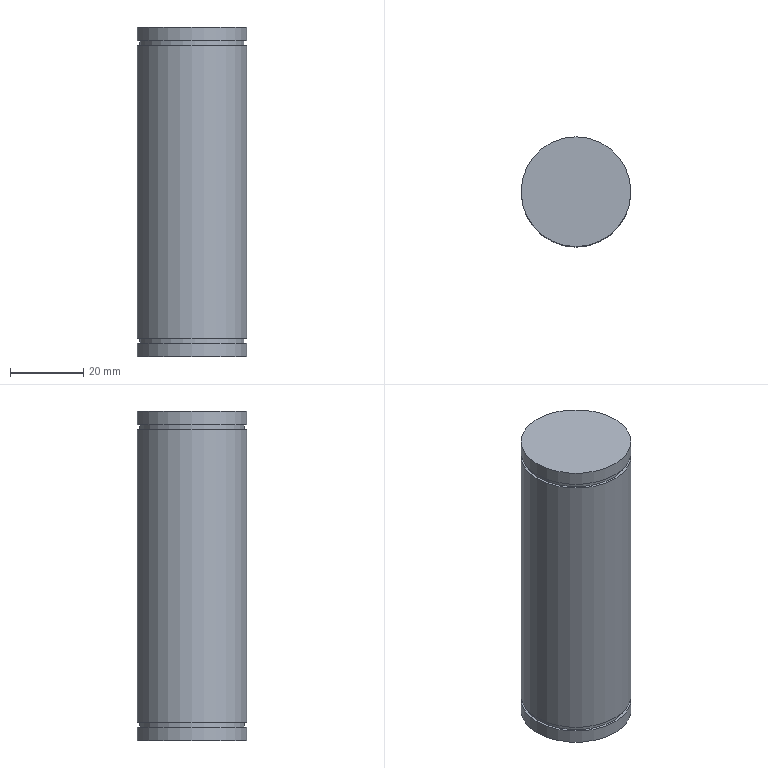Part | NX | features DATUM_CSYS 2, SKETCH 1, SWP104 1 | 1 solid | 11 faces | box 30 x 30 x 90 mm | volume 63450 mm3 | plane 6 | cylinder 5 | commonest cylinder face diameters 30 x3 28.6 x2
STEP:
#1=CARTESIAN_POINT('',(-15.,0.,5.));
#2=VERTEX_POINT('',#1);
#3=CARTESIAN_POINT('',(0.,0.,5.));
#4=DIRECTION('',(0.,0.,-1.));
#5=DIRECTION('',(-1.,0.,0.));
#6=AXIS2_PLACEMENT_3D('',#3,#4,#5);
#7=CIRCLE('',#6,15.);
#8=EDGE_CURVE('',#2,#2,#7,.T.);
#9=ORIENTED_EDGE('',*,*,#8,.F.);
#10=EDGE_LOOP('',(#9));
#11=FACE_BOUND('',#10,.T.);
#12=CARTESIAN_POINT('',(-15.,0.,85.));
#13=VERTEX_POINT('',#12);
#14=CARTESIAN_POINT('',(0.,0.,85.));
#15=DIRECTION('',(0.,0.,-1.));
#16=DIRECTION('',(-1.,0.,0.));
#17=AXIS2_PLACEMENT_3D('',#14,#15,#16);
#18=CIRCLE('',#17,15.);
#19=EDGE_CURVE('',#13,#13,#18,.T.);
#20=ORIENTED_EDGE('',*,*,#19,.T.);
#21=EDGE_LOOP('',(#20));
#22=FACE_BOUND('',#21,.T.);
#23=CARTESIAN_POINT('',(0.,0.,0.));
#24=DIRECTION('',(0.,0.,-1.));
#25=DIRECTION('',(-1.,0.,0.));
#26=AXIS2_PLACEMENT_3D('',#23,#24,#25);
#27=CYLINDRICAL_SURFACE('',#26,15.);
#28=ADVANCED_FACE('',(#11,#22),#27,.T.);
#29=CARTESIAN_POINT('',(-14.3,0.,5.));
#30=VERTEX_POINT('',#29);
#31=CARTESIAN_POINT('',(0.,0.,5.));
#32=DIRECTION('',(0.,0.,-1.));
#33=DIRECTION('',(-1.,0.,0.));
#34=AXIS2_PLACEMENT_3D('',#31,#32,#33);
#35=CIRCLE('',#34,14.3);
#36=EDGE_CURVE('',#30,#30,#35,.T.);
#37=ORIENTED_EDGE('',*,*,#36,.F.);
#38=EDGE_LOOP('',(#37));
#39=FACE_BOUND('',#38,.T.);
#40=ORIENTED_EDGE('',*,*,#8,.T.);
#41=EDGE_LOOP('',(#40));
#42=FACE_BOUND('',#41,.T.);
#43=CARTESIAN_POINT('',(0.,15.,5.));
#44=DIRECTION('',(0.,0.,1.));
#45=DIRECTION('',(1.,0.,0.));
#46=AXIS2_PLACEMENT_3D('',#43,#44,#45);
#47=PLANE('',#46);
#48=ADVANCED_FACE('',(#39,#42),#47,.F.);
#49=CARTESIAN_POINT('',(-14.3,0.,3.7));
#50=VERTEX_POINT('',#49);
#51=CARTESIAN_POINT('',(0.,0.,3.7));
#52=DIRECTION('',(0.,0.,-1.));
#53=DIRECTION('',(-1.,0.,0.));
#54=AXIS2_PLACEMENT_3D('',#51,#52,#53);
#55=CIRCLE('',#54,14.3);
#56=EDGE_CURVE('',#50,#50,#55,.T.);
#57=ORIENTED_EDGE('',*,*,#56,.F.);
#58=EDGE_LOOP('',(#57));
#59=FACE_BOUND('',#58,.T.);
#60=ORIENTED_EDGE('',*,*,#36,.T.);
#61=EDGE_LOOP('',(#60));
#62=FACE_BOUND('',#61,.T.);
#63=CARTESIAN_POINT('',(0.,0.,0.));
#64=DIRECTION('',(0.,0.,-1.));
#65=DIRECTION('',(-1.,0.,0.));
#66=AXIS2_PLACEMENT_3D('',#63,#64,#65);
#67=CYLINDRICAL_SURFACE('',#66,14.3);
#68=ADVANCED_FACE('',(#59,#62),#67,.T.);
#69=CARTESIAN_POINT('',(-15.,0.,3.7));
#70=VERTEX_POINT('',#69);
#71=CARTESIAN_POINT('',(0.,0.,3.7));
#72=DIRECTION('',(0.,0.,-1.));
#73=DIRECTION('',(-1.,0.,0.));
#74=AXIS2_PLACEMENT_3D('',#71,#72,#73);
#75=CIRCLE('',#74,15.);
#76=EDGE_CURVE('',#70,#70,#75,.T.);
#77=ORIENTED_EDGE('',*,*,#76,.F.);
#78=EDGE_LOOP('',(#77));
#79=FACE_BOUND('',#78,.T.);
#80=ORIENTED_EDGE('',*,*,#56,.T.);
#81=EDGE_LOOP('',(#80));
#82=FACE_BOUND('',#81,.T.);
#83=CARTESIAN_POINT('',(0.,14.3,3.7));
#84=DIRECTION('',(0.,0.,-1.));
#85=DIRECTION('',(-1.,0.,0.));
#86=AXIS2_PLACEMENT_3D('',#83,#84,#85);
#87=PLANE('',#86);
#88=ADVANCED_FACE('',(#79,#82),#87,.F.);
#89=CARTESIAN_POINT('',(-15.,0.,0.));
#90=VERTEX_POINT('',#89);
#91=CARTESIAN_POINT('',(0.,0.,0.));
#92=DIRECTION('',(0.,0.,-1.));
#93=DIRECTION('',(-1.,0.,0.));
#94=AXIS2_PLACEMENT_3D('',#91,#92,#93);
#95=CIRCLE('',#94,15.);
#96=EDGE_CURVE('',#90,#90,#95,.T.);
#97=ORIENTED_EDGE('',*,*,#96,.F.);
#98=EDGE_LOOP('',(#97));
#99=FACE_BOUND('',#98,.T.);
#100=ORIENTED_EDGE('',*,*,#76,.T.);
#101=EDGE_LOOP('',(#100));
#102=FACE_BOUND('',#101,.T.);
#103=CARTESIAN_POINT('',(0.,0.,0.));
#104=DIRECTION('',(0.,0.,-1.));
#105=DIRECTION('',(-1.,0.,0.));
#106=AXIS2_PLACEMENT_3D('',#103,#104,#105);
#107=CYLINDRICAL_SURFACE('',#106,15.);
#108=ADVANCED_FACE('',(#99,#102),#107,.T.);
#109=ORIENTED_EDGE('',*,*,#96,.T.);
#110=EDGE_LOOP('',(#109));
#111=FACE_BOUND('',#110,.T.);
#112=CARTESIAN_POINT('',(0.,15.,0.));
#113=DIRECTION('',(0.,0.,1.));
#114=DIRECTION('',(1.,0.,0.));
#115=AXIS2_PLACEMENT_3D('',#112,#113,#114);
#116=PLANE('',#115);
#117=ADVANCED_FACE('',(#111),#116,.F.);
#118=CARTESIAN_POINT('',(-15.,0.,90.));
#119=VERTEX_POINT('',#118);
#120=CARTESIAN_POINT('',(0.,0.,90.));
#121=DIRECTION('',(0.,0.,-1.));
#122=DIRECTION('',(-1.,0.,0.));
#123=AXIS2_PLACEMENT_3D('',#120,#121,#122);
#124=CIRCLE('',#123,15.);
#125=EDGE_CURVE('',#119,#119,#124,.T.);
#126=ORIENTED_EDGE('',*,*,#125,.F.);
#127=EDGE_LOOP('',(#126));
#128=FACE_BOUND('',#127,.T.);
#129=CARTESIAN_POINT('',(0.,0.,90.));
#130=DIRECTION('',(0.,0.,-1.));
#131=DIRECTION('',(-1.,0.,0.));
#132=AXIS2_PLACEMENT_3D('',#129,#130,#131);
#133=PLANE('',#132);
#134=ADVANCED_FACE('',(#128),#133,.F.);
#135=CARTESIAN_POINT('',(-15.,0.,86.3));
#136=VERTEX_POINT('',#135);
#137=CARTESIAN_POINT('',(0.,0.,86.3));
#138=DIRECTION('',(0.,0.,-1.));
#139=DIRECTION('',(-1.,0.,0.));
#140=AXIS2_PLACEMENT_3D('',#137,#138,#139);
#141=CIRCLE('',#140,15.);
#142=EDGE_CURVE('',#136,#136,#141,.T.);
#143=ORIENTED_EDGE('',*,*,#142,.F.);
#144=EDGE_LOOP('',(#143));
#145=FACE_BOUND('',#144,.T.);
#146=ORIENTED_EDGE('',*,*,#125,.T.);
#147=EDGE_LOOP('',(#146));
#148=FACE_BOUND('',#147,.T.);
#149=CARTESIAN_POINT('',(0.,0.,0.));
#150=DIRECTION('',(0.,0.,-1.));
#151=DIRECTION('',(-1.,0.,0.));
#152=AXIS2_PLACEMENT_3D('',#149,#150,#151);
#153=CYLINDRICAL_SURFACE('',#152,15.);
#154=ADVANCED_FACE('',(#145,#148),#153,.T.);
#155=CARTESIAN_POINT('',(-14.3,0.,86.3));
#156=VERTEX_POINT('',#155);
#157=CARTESIAN_POINT('',(0.,0.,86.3));
#158=DIRECTION('',(0.,0.,-1.));
#159=DIRECTION('',(-1.,0.,0.));
#160=AXIS2_PLACEMENT_3D('',#157,#158,#159);
#161=CIRCLE('',#160,14.3);
#162=EDGE_CURVE('',#156,#156,#161,.T.);
#163=ORIENTED_EDGE('',*,*,#162,.F.);
#164=EDGE_LOOP('',(#163));
#165=FACE_BOUND('',#164,.T.);
#166=ORIENTED_EDGE('',*,*,#142,.T.);
#167=EDGE_LOOP('',(#166));
#168=FACE_BOUND('',#167,.T.);
#169=CARTESIAN_POINT('',(0.,15.,86.3));
#170=DIRECTION('',(0.,0.,1.));
#171=DIRECTION('',(1.,0.,0.));
#172=AXIS2_PLACEMENT_3D('',#169,#170,#171);
#173=PLANE('',#172);
#174=ADVANCED_FACE('',(#165,#168),#173,.F.);
#175=CARTESIAN_POINT('',(-14.3,0.,85.));
#176=VERTEX_POINT('',#175);
#177=CARTESIAN_POINT('',(0.,0.,85.));
#178=DIRECTION('',(0.,0.,-1.));
#179=DIRECTION('',(-1.,0.,0.));
#180=AXIS2_PLACEMENT_3D('',#177,#178,#179);
#181=CIRCLE('',#180,14.3);
#182=EDGE_CURVE('',#176,#176,#181,.T.);
#183=ORIENTED_EDGE('',*,*,#182,.F.);
#184=EDGE_LOOP('',(#183));
#185=FACE_BOUND('',#184,.T.);
#186=ORIENTED_EDGE('',*,*,#162,.T.);
#187=EDGE_LOOP('',(#186));
#188=FACE_BOUND('',#187,.T.);
#189=CARTESIAN_POINT('',(0.,0.,0.));
#190=DIRECTION('',(0.,0.,-1.));
#191=DIRECTION('',(-1.,0.,0.));
#192=AXIS2_PLACEMENT_3D('',#189,#190,#191);
#193=CYLINDRICAL_SURFACE('',#192,14.3);
#194=ADVANCED_FACE('',(#185,#188),#193,.T.);
#195=ORIENTED_EDGE('',*,*,#19,.F.);
#196=EDGE_LOOP('',(#195));
#197=FACE_BOUND('',#196,.T.);
#198=ORIENTED_EDGE('',*,*,#182,.T.);
#199=EDGE_LOOP('',(#198));
#200=FACE_BOUND('',#199,.T.);
#201=CARTESIAN_POINT('',(0.,14.3,85.));
#202=DIRECTION('',(0.,0.,-1.));
#203=DIRECTION('',(-1.,0.,0.));
#204=AXIS2_PLACEMENT_3D('',#201,#202,#203);
#205=PLANE('',#204);
#206=ADVANCED_FACE('',(#197,#200),#205,.F.);
#207=CLOSED_SHELL('',(#28,#48,#68,#88,#108,#117,#134,#154,#174,#194,#206));
#208=MANIFOLD_SOLID_BREP('',#207);
#209=(LENGTH_UNIT()NAMED_UNIT(*)SI_UNIT(.MILLI.,.METRE.));
#210=UNCERTAINTY_MEASURE_WITH_UNIT(LENGTH_MEASURE(0.00001),#209,'','');
#211=(NAMED_UNIT(*)PLANE_ANGLE_UNIT()SI_UNIT($,.RADIAN.));
#212=(NAMED_UNIT(*)SI_UNIT($,.STERADIAN.)SOLID_ANGLE_UNIT());
#213=(GEOMETRIC_REPRESENTATION_CONTEXT(3)GLOBAL_UNCERTAINTY_ASSIGNED_CONTEXT((#210))GLOBAL_UNIT_ASSIGNED_CONTEXT((#209,#211,#212))REPRESENTATION_CONTEXT('',''));
#214=ADVANCED_BREP_SHAPE_REPRESENTATION('',(#208),#213);